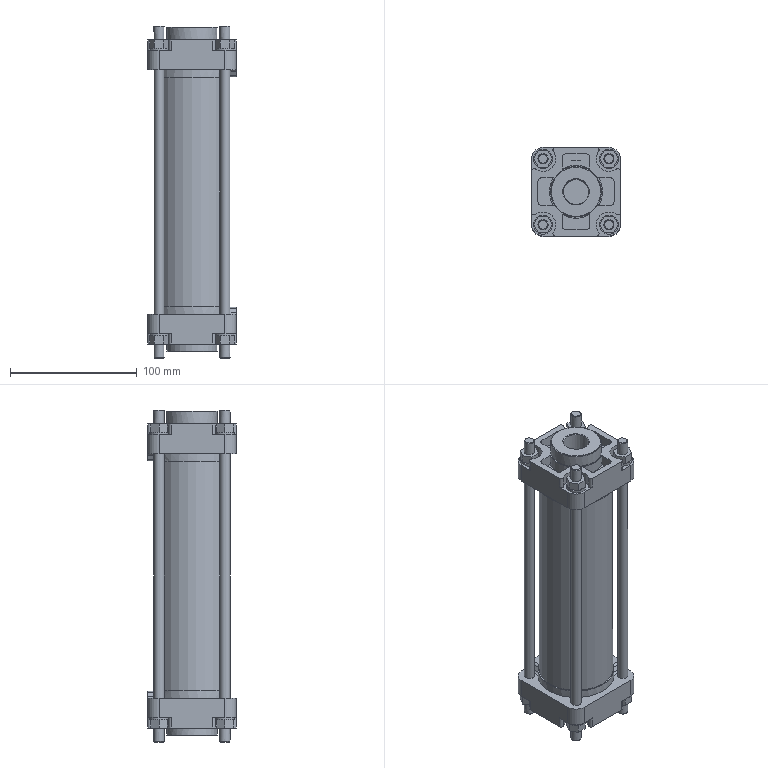Part | NX | features Hydraulic2.1_50 2 | 1 solid | 352 faces | box 70 x 70 x 262 mm | volume 413187 mm3 | plane 219 | cylinder 120 | cone 13 | commonest cylinder face diameters 4 x34 6 x16 5 x12 8 x12 20 x10 15 x8